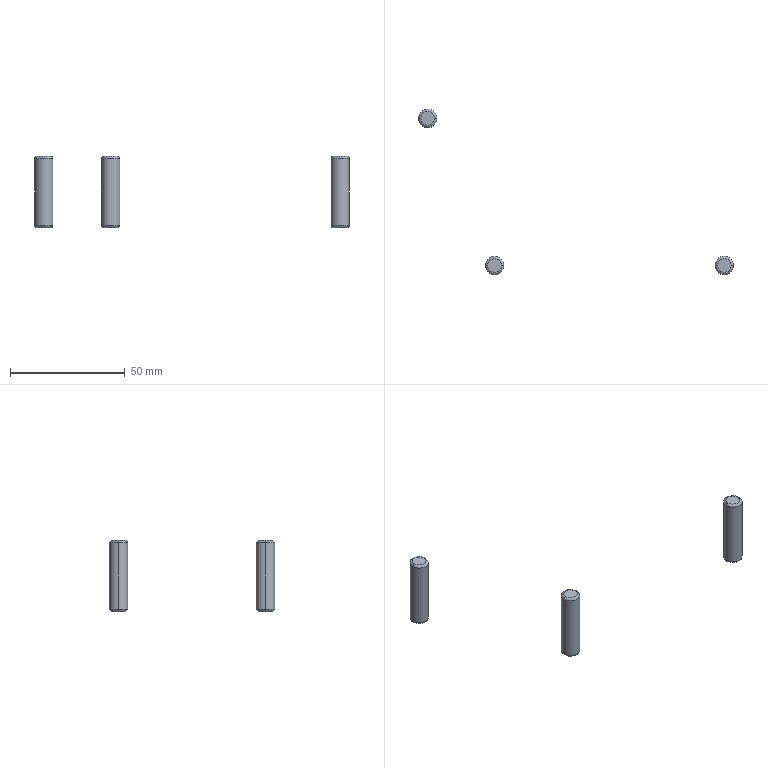Part | SolidWorks | features Fillet 3, Extrusion 1 | 3 solids | 24 faces | box 137.1 x 72.1 x 31 mm | volume 4644 mm3 | torus 12 | cylinder 6 | plane 6 | commonest cylinder face diameters 8 x6
STEP:
#1=CARTESIAN_POINT('',(-83.1,0.,25.));
#2=VERTEX_POINT('',#1);
#3=CARTESIAN_POINT('',(-75.1,0.,25.));
#4=VERTEX_POINT('',#3);
#5=CARTESIAN_POINT('',(-79.1,0.,25.));
#6=DIRECTION('',(0.,0.,-1.));
#7=DIRECTION('',(1.,0.,0.));
#8=AXIS2_PLACEMENT_3D('',#5,#6,#7);
#9=CIRCLE('',#8,4.);
#10=EDGE_CURVE('',#2,#4,#9,.T.);
#11=ORIENTED_EDGE('',*,*,#10,.F.);
#12=CARTESIAN_POINT('',(-82.1,0.,26.));
#13=VERTEX_POINT('',#12);
#14=CARTESIAN_POINT('',(-82.1,0.,25.));
#15=DIRECTION('',(0.,1.,0.));
#16=DIRECTION('',(-1.,0.,0.));
#17=AXIS2_PLACEMENT_3D('',#14,#15,#16);
#18=CIRCLE('',#17,1.);
#19=EDGE_CURVE('',#2,#13,#18,.T.);
#20=ORIENTED_EDGE('',*,*,#19,.T.);
#21=CARTESIAN_POINT('',(-76.1,0.,26.));
#22=VERTEX_POINT('',#21);
#23=CARTESIAN_POINT('',(-79.1,0.,26.));
#24=DIRECTION('',(0.,0.,1.));
#25=DIRECTION('',(1.,0.,0.));
#26=AXIS2_PLACEMENT_3D('',#23,#24,#25);
#27=CIRCLE('',#26,3.);
#28=EDGE_CURVE('',#22,#13,#27,.T.);
#29=ORIENTED_EDGE('',*,*,#28,.F.);
#30=CARTESIAN_POINT('',(-76.1,0.,25.));
#31=DIRECTION('',(0.,-1.,0.));
#32=DIRECTION('',(0.,0.,-1.));
#33=AXIS2_PLACEMENT_3D('',#30,#31,#32);
#34=CIRCLE('',#33,1.);
#35=EDGE_CURVE('',#4,#22,#34,.T.);
#36=ORIENTED_EDGE('',*,*,#35,.F.);
#37=EDGE_LOOP('',(#11,#20,#29,#36));
#38=FACE_OUTER_BOUND('',#37,.T.);
#39=CARTESIAN_POINT('',(-79.1,0.,25.));
#40=DIRECTION('',(0.,0.,1.));
#41=DIRECTION('',(1.,0.,0.));
#42=AXIS2_PLACEMENT_3D('',#39,#40,#41);
#43=TOROIDAL_SURFACE('',#42,3.,1.);
#44=ADVANCED_FACE('',(#38),#43,.T.);
#45=CARTESIAN_POINT('',(-75.1,0.,-4.));
#46=VERTEX_POINT('',#45);
#47=CARTESIAN_POINT('',(-83.1,0.,-4.));
#48=VERTEX_POINT('',#47);
#49=CARTESIAN_POINT('',(-79.1,0.,-4.));
#50=DIRECTION('',(0.,0.,1.));
#51=DIRECTION('',(-1.,0.,0.));
#52=AXIS2_PLACEMENT_3D('',#49,#50,#51);
#53=CIRCLE('',#52,4.);
#54=EDGE_CURVE('',#46,#48,#53,.T.);
#55=ORIENTED_EDGE('',*,*,#54,.F.);
#56=CARTESIAN_POINT('',(-76.1,0.,-5.));
#57=VERTEX_POINT('',#56);
#58=CARTESIAN_POINT('',(-76.1,0.,-4.));
#59=DIRECTION('',(0.,1.,0.));
#60=DIRECTION('',(-1.,0.,0.));
#61=AXIS2_PLACEMENT_3D('',#58,#59,#60);
#62=CIRCLE('',#61,1.);
#63=EDGE_CURVE('',#46,#57,#62,.T.);
#64=ORIENTED_EDGE('',*,*,#63,.T.);
#65=CARTESIAN_POINT('',(-82.1,0.,-5.));
#66=VERTEX_POINT('',#65);
#67=CARTESIAN_POINT('',(-79.1,0.,-5.));
#68=DIRECTION('',(0.,0.,-1.));
#69=DIRECTION('',(-1.,0.,0.));
#70=AXIS2_PLACEMENT_3D('',#67,#68,#69);
#71=CIRCLE('',#70,3.);
#72=EDGE_CURVE('',#66,#57,#71,.T.);
#73=ORIENTED_EDGE('',*,*,#72,.F.);
#74=CARTESIAN_POINT('',(-82.1,0.,-4.));
#75=DIRECTION('',(0.,-1.,0.));
#76=DIRECTION('',(0.,0.,-1.));
#77=AXIS2_PLACEMENT_3D('',#74,#75,#76);
#78=CIRCLE('',#77,1.);
#79=EDGE_CURVE('',#48,#66,#78,.T.);
#80=ORIENTED_EDGE('',*,*,#79,.F.);
#81=EDGE_LOOP('',(#55,#64,#73,#80));
#82=FACE_OUTER_BOUND('',#81,.T.);
#83=CARTESIAN_POINT('',(-79.1,0.,-4.));
#84=DIRECTION('',(0.,0.,-1.));
#85=DIRECTION('',(-1.,0.,0.));
#86=AXIS2_PLACEMENT_3D('',#83,#84,#85);
#87=TOROIDAL_SURFACE('',#86,3.,1.);
#88=ADVANCED_FACE('',(#82),#87,.T.);
#89=ORIENTED_EDGE('',*,*,#54,.T.);
#90=CARTESIAN_POINT('',(-83.1,0.,-16.314));
#91=DIRECTION('',(0.,0.,1.));
#92=VECTOR('',#91,1000.);
#93=LINE('',#90,#92);
#94=EDGE_CURVE('',#48,#2,#93,.T.);
#95=ORIENTED_EDGE('',*,*,#94,.T.);
#96=ORIENTED_EDGE('',*,*,#10,.T.);
#97=CARTESIAN_POINT('',(-75.1,0.,-16.314));
#98=DIRECTION('',(0.,0.,1.));
#99=VECTOR('',#98,1000.);
#100=LINE('',#97,#99);
#101=EDGE_CURVE('',#46,#4,#100,.T.);
#102=ORIENTED_EDGE('',*,*,#101,.F.);
#103=EDGE_LOOP('',(#89,#95,#96,#102));
#104=FACE_OUTER_BOUND('',#103,.T.);
#105=CARTESIAN_POINT('',(-79.1,0.,-16.314));
#106=DIRECTION('',(0.,0.,1.));
#107=DIRECTION('',(1.,0.,0.));
#108=AXIS2_PLACEMENT_3D('',#105,#106,#107);
#109=CYLINDRICAL_SURFACE('',#108,4.);
#110=ADVANCED_FACE('',(#104),#109,.T.);
#111=ORIENTED_EDGE('',*,*,#94,.F.);
#112=CARTESIAN_POINT('',(-79.1,0.,-4.));
#113=DIRECTION('',(0.,0.,1.));
#114=DIRECTION('',(-1.,0.,0.));
#115=AXIS2_PLACEMENT_3D('',#112,#113,#114);
#116=CIRCLE('',#115,4.);
#117=EDGE_CURVE('',#48,#46,#116,.T.);
#118=ORIENTED_EDGE('',*,*,#117,.T.);
#119=ORIENTED_EDGE('',*,*,#101,.T.);
#120=CARTESIAN_POINT('',(-79.1,0.,25.));
#121=DIRECTION('',(0.,0.,-1.));
#122=DIRECTION('',(1.,0.,0.));
#123=AXIS2_PLACEMENT_3D('',#120,#121,#122);
#124=CIRCLE('',#123,4.);
#125=EDGE_CURVE('',#4,#2,#124,.T.);
#126=ORIENTED_EDGE('',*,*,#125,.T.);
#127=EDGE_LOOP('',(#111,#118,#119,#126));
#128=FACE_OUTER_BOUND('',#127,.T.);
#129=CARTESIAN_POINT('',(-79.1,0.,-16.314));
#130=DIRECTION('',(0.,0.,1.));
#131=DIRECTION('',(1.,0.,0.));
#132=AXIS2_PLACEMENT_3D('',#129,#130,#131);
#133=CYLINDRICAL_SURFACE('',#132,4.);
#134=ADVANCED_FACE('',(#128),#133,.T.);
#135=ORIENTED_EDGE('',*,*,#72,.T.);
#136=CARTESIAN_POINT('',(-79.1,0.,-5.));
#137=DIRECTION('',(0.,0.,-1.));
#138=DIRECTION('',(-1.,0.,0.));
#139=AXIS2_PLACEMENT_3D('',#136,#137,#138);
#140=CIRCLE('',#139,3.);
#141=EDGE_CURVE('',#57,#66,#140,.T.);
#142=ORIENTED_EDGE('',*,*,#141,.T.);
#143=EDGE_LOOP('',(#135,#142));
#144=FACE_OUTER_BOUND('',#143,.T.);
#145=CARTESIAN_POINT('',(-79.1,0.,-5.));
#146=DIRECTION('',(0.,0.,-1.));
#147=DIRECTION('',(-1.,0.,0.));
#148=AXIS2_PLACEMENT_3D('',#145,#146,#147);
#149=PLANE('',#148);
#150=ADVANCED_FACE('',(#144),#149,.T.);
#151=ORIENTED_EDGE('',*,*,#28,.T.);
#152=CARTESIAN_POINT('',(-79.1,0.,26.));
#153=DIRECTION('',(0.,0.,1.));
#154=DIRECTION('',(1.,0.,0.));
#155=AXIS2_PLACEMENT_3D('',#152,#153,#154);
#156=CIRCLE('',#155,3.);
#157=EDGE_CURVE('',#13,#22,#156,.T.);
#158=ORIENTED_EDGE('',*,*,#157,.T.);
#159=EDGE_LOOP('',(#151,#158));
#160=FACE_OUTER_BOUND('',#159,.T.);
#161=CARTESIAN_POINT('',(-79.1,0.,26.));
#162=DIRECTION('',(0.,0.,1.));
#163=DIRECTION('',(1.,0.,0.));
#164=AXIS2_PLACEMENT_3D('',#161,#162,#163);
#165=PLANE('',#164);
#166=ADVANCED_FACE('',(#160),#165,.T.);
#167=ORIENTED_EDGE('',*,*,#63,.F.);
#168=ORIENTED_EDGE('',*,*,#117,.F.);
#169=ORIENTED_EDGE('',*,*,#79,.T.);
#170=ORIENTED_EDGE('',*,*,#141,.F.);
#171=EDGE_LOOP('',(#167,#168,#169,#170));
#172=FACE_OUTER_BOUND('',#171,.T.);
#173=CARTESIAN_POINT('',(-79.1,0.,-4.));
#174=DIRECTION('',(0.,0.,-1.));
#175=DIRECTION('',(-1.,0.,0.));
#176=AXIS2_PLACEMENT_3D('',#173,#174,#175);
#177=TOROIDAL_SURFACE('',#176,3.,1.);
#178=ADVANCED_FACE('',(#172),#177,.T.);
#179=ORIENTED_EDGE('',*,*,#19,.F.);
#180=ORIENTED_EDGE('',*,*,#125,.F.);
#181=ORIENTED_EDGE('',*,*,#35,.T.);
#182=ORIENTED_EDGE('',*,*,#157,.F.);
#183=EDGE_LOOP('',(#179,#180,#181,#182));
#184=FACE_OUTER_BOUND('',#183,.T.);
#185=CARTESIAN_POINT('',(-79.1,0.,25.));
#186=DIRECTION('',(0.,0.,1.));
#187=DIRECTION('',(1.,0.,0.));
#188=AXIS2_PLACEMENT_3D('',#185,#186,#187);
#189=TOROIDAL_SURFACE('',#188,3.,1.);
#190=ADVANCED_FACE('',(#184),#189,.T.);
#191=CLOSED_SHELL('',(#44,#88,#110,#134,#150,#166,#178,#190));
#192=MANIFOLD_SOLID_BREP('',#191);
#193=CARTESIAN_POINT('',(-46.,-64.1,-4.));
#194=VERTEX_POINT('',#193);
#195=CARTESIAN_POINT('',(-54.,-64.1,-4.));
#196=VERTEX_POINT('',#195);
#197=CARTESIAN_POINT('',(-50.,-64.1,-4.));
#198=DIRECTION('',(0.,0.,1.));
#199=DIRECTION('',(-1.,0.,0.));
#200=AXIS2_PLACEMENT_3D('',#197,#198,#199);
#201=CIRCLE('',#200,4.);
#202=EDGE_CURVE('',#194,#196,#201,.T.);
#203=ORIENTED_EDGE('',*,*,#202,.F.);
#204=CARTESIAN_POINT('',(-47.,-64.1,-5.));
#205=VERTEX_POINT('',#204);
#206=CARTESIAN_POINT('',(-47.,-64.1,-4.));
#207=DIRECTION('',(0.,1.,0.));
#208=DIRECTION('',(-1.,0.,0.));
#209=AXIS2_PLACEMENT_3D('',#206,#207,#208);
#210=CIRCLE('',#209,1.);
#211=EDGE_CURVE('',#194,#205,#210,.T.);
#212=ORIENTED_EDGE('',*,*,#211,.T.);
#213=CARTESIAN_POINT('',(-53.,-64.1,-5.));
#214=VERTEX_POINT('',#213);
#215=CARTESIAN_POINT('',(-50.,-64.1,-5.));
#216=DIRECTION('',(0.,0.,-1.));
#217=DIRECTION('',(-1.,0.,0.));
#218=AXIS2_PLACEMENT_3D('',#215,#216,#217);
#219=CIRCLE('',#218,3.);
#220=EDGE_CURVE('',#214,#205,#219,.T.);
#221=ORIENTED_EDGE('',*,*,#220,.F.);
#222=CARTESIAN_POINT('',(-53.,-64.1,-4.));
#223=DIRECTION('',(0.,-1.,0.));
#224=DIRECTION('',(0.,0.,-1.));
#225=AXIS2_PLACEMENT_3D('',#222,#223,#224);
#226=CIRCLE('',#225,1.);
#227=EDGE_CURVE('',#196,#214,#226,.T.);
#228=ORIENTED_EDGE('',*,*,#227,.F.);
#229=EDGE_LOOP('',(#203,#212,#221,#228));
#230=FACE_OUTER_BOUND('',#229,.T.);
#231=CARTESIAN_POINT('',(-50.,-64.1,-4.));
#232=DIRECTION('',(0.,0.,-1.));
#233=DIRECTION('',(-1.,0.,0.));
#234=AXIS2_PLACEMENT_3D('',#231,#232,#233);
#235=TOROIDAL_SURFACE('',#234,3.,1.);
#236=ADVANCED_FACE('',(#230),#235,.T.);
#237=CARTESIAN_POINT('',(-54.,-64.1,25.));
#238=VERTEX_POINT('',#237);
#239=CARTESIAN_POINT('',(-46.,-64.1,25.));
#240=VERTEX_POINT('',#239);
#241=CARTESIAN_POINT('',(-50.,-64.1,25.));
#242=DIRECTION('',(0.,0.,-1.));
#243=DIRECTION('',(1.,0.,0.));
#244=AXIS2_PLACEMENT_3D('',#241,#242,#243);
#245=CIRCLE('',#244,4.);
#246=EDGE_CURVE('',#238,#240,#245,.T.);
#247=ORIENTED_EDGE('',*,*,#246,.F.);
#248=CARTESIAN_POINT('',(-53.,-64.1,26.));
#249=VERTEX_POINT('',#248);
#250=CARTESIAN_POINT('',(-53.,-64.1,25.));
#251=DIRECTION('',(0.,1.,0.));
#252=DIRECTION('',(-1.,0.,0.));
#253=AXIS2_PLACEMENT_3D('',#250,#251,#252);
#254=CIRCLE('',#253,1.);
#255=EDGE_CURVE('',#238,#249,#254,.T.);
#256=ORIENTED_EDGE('',*,*,#255,.T.);
#257=CARTESIAN_POINT('',(-47.,-64.1,26.));
#258=VERTEX_POINT('',#257);
#259=CARTESIAN_POINT('',(-50.,-64.1,26.));
#260=DIRECTION('',(0.,0.,1.));
#261=DIRECTION('',(1.,0.,0.));
#262=AXIS2_PLACEMENT_3D('',#259,#260,#261);
#263=CIRCLE('',#262,3.);
#264=EDGE_CURVE('',#258,#249,#263,.T.);
#265=ORIENTED_EDGE('',*,*,#264,.F.);
#266=CARTESIAN_POINT('',(-47.,-64.1,25.));
#267=DIRECTION('',(0.,-1.,0.));
#268=DIRECTION('',(0.,0.,-1.));
#269=AXIS2_PLACEMENT_3D('',#266,#267,#268);
#270=CIRCLE('',#269,1.);
#271=EDGE_CURVE('',#240,#258,#270,.T.);
#272=ORIENTED_EDGE('',*,*,#271,.F.);
#273=EDGE_LOOP('',(#247,#256,#265,#272));
#274=FACE_OUTER_BOUND('',#273,.T.);
#275=CARTESIAN_POINT('',(-50.,-64.1,25.));
#276=DIRECTION('',(0.,0.,1.));
#277=DIRECTION('',(1.,0.,0.));
#278=AXIS2_PLACEMENT_3D('',#275,#276,#277);
#279=TOROIDAL_SURFACE('',#278,3.,1.);
#280=ADVANCED_FACE('',(#274),#279,.T.);
#281=ORIENTED_EDGE('',*,*,#202,.T.);
#282=CARTESIAN_POINT('',(-54.,-64.1,-16.314));
#283=DIRECTION('',(0.,0.,1.));
#284=VECTOR('',#283,1000.);
#285=LINE('',#282,#284);
#286=EDGE_CURVE('',#196,#238,#285,.T.);
#287=ORIENTED_EDGE('',*,*,#286,.T.);
#288=ORIENTED_EDGE('',*,*,#246,.T.);
#289=CARTESIAN_POINT('',(-46.,-64.1,-16.314));
#290=DIRECTION('',(0.,0.,1.));
#291=VECTOR('',#290,1000.);
#292=LINE('',#289,#291);
#293=EDGE_CURVE('',#194,#240,#292,.T.);
#294=ORIENTED_EDGE('',*,*,#293,.F.);
#295=EDGE_LOOP('',(#281,#287,#288,#294));
#296=FACE_OUTER_BOUND('',#295,.T.);
#297=CARTESIAN_POINT('',(-50.,-64.1,-16.314));
#298=DIRECTION('',(0.,0.,1.));
#299=DIRECTION('',(1.,0.,0.));
#300=AXIS2_PLACEMENT_3D('',#297,#298,#299);
#301=CYLINDRICAL_SURFACE('',#300,4.);
#302=ADVANCED_FACE('',(#296),#301,.T.);
#303=ORIENTED_EDGE('',*,*,#220,.T.);
#304=CARTESIAN_POINT('',(-50.,-64.1,-5.));
#305=DIRECTION('',(0.,0.,-1.));
#306=DIRECTION('',(-1.,0.,0.));
#307=AXIS2_PLACEMENT_3D('',#304,#305,#306);
#308=CIRCLE('',#307,3.);
#309=EDGE_CURVE('',#205,#214,#308,.T.);
#310=ORIENTED_EDGE('',*,*,#309,.T.);
#311=EDGE_LOOP('',(#303,#310));
#312=FACE_OUTER_BOUND('',#311,.T.);
#313=CARTESIAN_POINT('',(-79.1,0.,-5.));
#314=DIRECTION('',(0.,0.,-1.));
#315=DIRECTION('',(-1.,0.,0.));
#316=AXIS2_PLACEMENT_3D('',#313,#314,#315);
#317=PLANE('',#316);
#318=ADVANCED_FACE('',(#312),#317,.T.);
#319=ORIENTED_EDGE('',*,*,#286,.F.);
#320=CARTESIAN_POINT('',(-50.,-64.1,-4.));
#321=DIRECTION('',(0.,0.,1.));
#322=DIRECTION('',(-1.,0.,0.));
#323=AXIS2_PLACEMENT_3D('',#320,#321,#322);
#324=CIRCLE('',#323,4.);
#325=EDGE_CURVE('',#196,#194,#324,.T.);
#326=ORIENTED_EDGE('',*,*,#325,.T.);
#327=ORIENTED_EDGE('',*,*,#293,.T.);
#328=CARTESIAN_POINT('',(-50.,-64.1,25.));
#329=DIRECTION('',(0.,0.,-1.));
#330=DIRECTION('',(1.,0.,0.));
#331=AXIS2_PLACEMENT_3D('',#328,#329,#330);
#332=CIRCLE('',#331,4.);
#333=EDGE_CURVE('',#240,#238,#332,.T.);
#334=ORIENTED_EDGE('',*,*,#333,.T.);
#335=EDGE_LOOP('',(#319,#326,#327,#334));
#336=FACE_OUTER_BOUND('',#335,.T.);
#337=CARTESIAN_POINT('',(-50.,-64.1,-16.314));
#338=DIRECTION('',(0.,0.,1.));
#339=DIRECTION('',(1.,0.,0.));
#340=AXIS2_PLACEMENT_3D('',#337,#338,#339);
#341=CYLINDRICAL_SURFACE('',#340,4.);
#342=ADVANCED_FACE('',(#336),#341,.T.);
#343=ORIENTED_EDGE('',*,*,#264,.T.);
#344=CARTESIAN_POINT('',(-50.,-64.1,26.));
#345=DIRECTION('',(0.,0.,1.));
#346=DIRECTION('',(1.,0.,0.));
#347=AXIS2_PLACEMENT_3D('',#344,#345,#346);
#348=CIRCLE('',#347,3.);
#349=EDGE_CURVE('',#249,#258,#348,.T.);
#350=ORIENTED_EDGE('',*,*,#349,.T.);
#351=EDGE_LOOP('',(#343,#350));
#352=FACE_OUTER_BOUND('',#351,.T.);
#353=CARTESIAN_POINT('',(-50.,-64.1,26.));
#354=DIRECTION('',(0.,0.,1.));
#355=DIRECTION('',(1.,0.,0.));
#356=AXIS2_PLACEMENT_3D('',#353,#354,#355);
#357=PLANE('',#356);
#358=ADVANCED_FACE('',(#352),#357,.T.);
#359=ORIENTED_EDGE('',*,*,#255,.F.);
#360=ORIENTED_EDGE('',*,*,#333,.F.);
#361=ORIENTED_EDGE('',*,*,#271,.T.);
#362=ORIENTED_EDGE('',*,*,#349,.F.);
#363=EDGE_LOOP('',(#359,#360,#361,#362));
#364=FACE_OUTER_BOUND('',#363,.T.);
#365=CARTESIAN_POINT('',(-50.,-64.1,25.));
#366=DIRECTION('',(0.,0.,1.));
#367=DIRECTION('',(1.,0.,0.));
#368=AXIS2_PLACEMENT_3D('',#365,#366,#367);
#369=TOROIDAL_SURFACE('',#368,3.,1.);
#370=ADVANCED_FACE('',(#364),#369,.T.);
#371=ORIENTED_EDGE('',*,*,#211,.F.);
#372=ORIENTED_EDGE('',*,*,#325,.F.);
#373=ORIENTED_EDGE('',*,*,#227,.T.);
#374=ORIENTED_EDGE('',*,*,#309,.F.);
#375=EDGE_LOOP('',(#371,#372,#373,#374));
#376=FACE_OUTER_BOUND('',#375,.T.);
#377=CARTESIAN_POINT('',(-50.,-64.1,-4.));
#378=DIRECTION('',(0.,0.,-1.));
#379=DIRECTION('',(-1.,0.,0.));
#380=AXIS2_PLACEMENT_3D('',#377,#378,#379);
#381=TOROIDAL_SURFACE('',#380,3.,1.);
#382=ADVANCED_FACE('',(#376),#381,.T.);
#383=CLOSED_SHELL('',(#236,#280,#302,#318,#342,#358,#370,#382));
#384=MANIFOLD_SOLID_BREP('',#383);
#385=CARTESIAN_POINT('',(46.,-64.1,25.));
#386=VERTEX_POINT('',#385);
#387=CARTESIAN_POINT('',(54.,-64.1,25.));
#388=VERTEX_POINT('',#387);
#389=CARTESIAN_POINT('',(50.,-64.1,25.));
#390=DIRECTION('',(0.,0.,-1.));
#391=DIRECTION('',(1.,0.,0.));
#392=AXIS2_PLACEMENT_3D('',#389,#390,#391);
#393=CIRCLE('',#392,4.);
#394=EDGE_CURVE('',#386,#388,#393,.T.);
#395=ORIENTED_EDGE('',*,*,#394,.F.);
#396=CARTESIAN_POINT('',(47.,-64.1,26.));
#397=VERTEX_POINT('',#396);
#398=CARTESIAN_POINT('',(47.,-64.1,25.));
#399=DIRECTION('',(0.,1.,0.));
#400=DIRECTION('',(-1.,0.,0.));
#401=AXIS2_PLACEMENT_3D('',#398,#399,#400);
#402=CIRCLE('',#401,1.);
#403=EDGE_CURVE('',#386,#397,#402,.T.);
#404=ORIENTED_EDGE('',*,*,#403,.T.);
#405=CARTESIAN_POINT('',(53.,-64.1,26.));
#406=VERTEX_POINT('',#405);
#407=CARTESIAN_POINT('',(50.,-64.1,26.));
#408=DIRECTION('',(0.,0.,1.));
#409=DIRECTION('',(1.,0.,0.));
#410=AXIS2_PLACEMENT_3D('',#407,#408,#409);
#411=CIRCLE('',#410,3.);
#412=EDGE_CURVE('',#406,#397,#411,.T.);
#413=ORIENTED_EDGE('',*,*,#412,.F.);
#414=CARTESIAN_POINT('',(53.,-64.1,25.));
#415=DIRECTION('',(0.,-1.,0.));
#416=DIRECTION('',(0.,0.,-1.));
#417=AXIS2_PLACEMENT_3D('',#414,#415,#416);
#418=CIRCLE('',#417,1.);
#419=EDGE_CURVE('',#388,#406,#418,.T.);
#420=ORIENTED_EDGE('',*,*,#419,.F.);
#421=EDGE_LOOP('',(#395,#404,#413,#420));
#422=FACE_OUTER_BOUND('',#421,.T.);
#423=CARTESIAN_POINT('',(50.,-64.1,25.));
#424=DIRECTION('',(0.,0.,1.));
#425=DIRECTION('',(1.,0.,0.));
#426=AXIS2_PLACEMENT_3D('',#423,#424,#425);
#427=TOROIDAL_SURFACE('',#426,3.,1.);
#428=ADVANCED_FACE('',(#422),#427,.T.);
#429=CARTESIAN_POINT('',(54.,-64.1,-4.));
#430=VERTEX_POINT('',#429);
#431=CARTESIAN_POINT('',(46.,-64.1,-4.));
#432=VERTEX_POINT('',#431);
#433=CARTESIAN_POINT('',(50.,-64.1,-4.));
#434=DIRECTION('',(0.,0.,1.));
#435=DIRECTION('',(-1.,0.,0.));
#436=AXIS2_PLACEMENT_3D('',#433,#434,#435);
#437=CIRCLE('',#436,4.);
#438=EDGE_CURVE('',#430,#432,#437,.T.);
#439=ORIENTED_EDGE('',*,*,#438,.F.);
#440=CARTESIAN_POINT('',(53.,-64.1,-5.));
#441=VERTEX_POINT('',#440);
#442=CARTESIAN_POINT('',(53.,-64.1,-4.));
#443=DIRECTION('',(0.,1.,0.));
#444=DIRECTION('',(-1.,0.,0.));
#445=AXIS2_PLACEMENT_3D('',#442,#443,#444);
#446=CIRCLE('',#445,1.);
#447=EDGE_CURVE('',#430,#441,#446,.T.);
#448=ORIENTED_EDGE('',*,*,#447,.T.);
#449=CARTESIAN_POINT('',(47.,-64.1,-5.));
#450=VERTEX_POINT('',#449);
#451=CARTESIAN_POINT('',(50.,-64.1,-5.));
#452=DIRECTION('',(0.,0.,-1.));
#453=DIRECTION('',(-1.,0.,0.));
#454=AXIS2_PLACEMENT_3D('',#451,#452,#453);
#455=CIRCLE('',#454,3.);
#456=EDGE_CURVE('',#450,#441,#455,.T.);
#457=ORIENTED_EDGE('',*,*,#456,.F.);
#458=CARTESIAN_POINT('',(47.,-64.1,-4.));
#459=DIRECTION('',(0.,-1.,0.));
#460=DIRECTION('',(0.,0.,-1.));
#461=AXIS2_PLACEMENT_3D('',#458,#459,#460);
#462=CIRCLE('',#461,1.);
#463=EDGE_CURVE('',#432,#450,#462,.T.);
#464=ORIENTED_EDGE('',*,*,#463,.F.);
#465=EDGE_LOOP('',(#439,#448,#457,#464));
#466=FACE_OUTER_BOUND('',#465,.T.);
#467=CARTESIAN_POINT('',(50.,-64.1,-4.));
#468=DIRECTION('',(0.,0.,-1.));
#469=DIRECTION('',(-1.,0.,0.));
#470=AXIS2_PLACEMENT_3D('',#467,#468,#469);
#471=TOROIDAL_SURFACE('',#470,3.,1.);
#472=ADVANCED_FACE('',(#466),#471,.T.);
#473=ORIENTED_EDGE('',*,*,#438,.T.);
#474=CARTESIAN_POINT('',(46.,-64.1,-16.314));
#475=DIRECTION('',(0.,0.,1.));
#476=VECTOR('',#475,1000.);
#477=LINE('',#474,#476);
#478=EDGE_CURVE('',#432,#386,#477,.T.);
#479=ORIENTED_EDGE('',*,*,#478,.T.);
#480=ORIENTED_EDGE('',*,*,#394,.T.);
#481=CARTESIAN_POINT('',(54.,-64.1,-16.314));
#482=DIRECTION('',(0.,0.,1.));
#483=VECTOR('',#482,1000.);
#484=LINE('',#481,#483);
#485=EDGE_CURVE('',#430,#388,#484,.T.);
#486=ORIENTED_EDGE('',*,*,#485,.F.);
#487=EDGE_LOOP('',(#473,#479,#480,#486));
#488=FACE_OUTER_BOUND('',#487,.T.);
#489=CARTESIAN_POINT('',(50.,-64.1,-16.314));
#490=DIRECTION('',(0.,0.,1.));
#491=DIRECTION('',(1.,0.,0.));
#492=AXIS2_PLACEMENT_3D('',#489,#490,#491);
#493=CYLINDRICAL_SURFACE('',#492,4.);
#494=ADVANCED_FACE('',(#488),#493,.T.);
#495=ORIENTED_EDGE('',*,*,#456,.T.);
#496=CARTESIAN_POINT('',(50.,-64.1,-5.));
#497=DIRECTION('',(0.,0.,-1.));
#498=DIRECTION('',(-1.,0.,0.));
#499=AXIS2_PLACEMENT_3D('',#496,#497,#498);
#500=CIRCLE('',#499,3.);
#501=EDGE_CURVE('',#441,#450,#500,.T.);
#502=ORIENTED_EDGE('',*,*,#501,.T.);
#503=EDGE_LOOP('',(#495,#502));
#504=FACE_OUTER_BOUND('',#503,.T.);
#505=CARTESIAN_POINT('',(-79.1,0.,-5.));
#506=DIRECTION('',(0.,0.,-1.));
#507=DIRECTION('',(-1.,0.,0.));
#508=AXIS2_PLACEMENT_3D('',#505,#506,#507);
#509=PLANE('',#508);
#510=ADVANCED_FACE('',(#504),#509,.T.);
#511=ORIENTED_EDGE('',*,*,#478,.F.);
#512=CARTESIAN_POINT('',(50.,-64.1,-4.));
#513=DIRECTION('',(0.,0.,1.));
#514=DIRECTION('',(-1.,0.,0.));
#515=AXIS2_PLACEMENT_3D('',#512,#513,#514);
#516=CIRCLE('',#515,4.);
#517=EDGE_CURVE('',#432,#430,#516,.T.);
#518=ORIENTED_EDGE('',*,*,#517,.T.);
#519=ORIENTED_EDGE('',*,*,#485,.T.);
#520=CARTESIAN_POINT('',(50.,-64.1,25.));
#521=DIRECTION('',(0.,0.,-1.));
#522=DIRECTION('',(1.,0.,0.));
#523=AXIS2_PLACEMENT_3D('',#520,#521,#522);
#524=CIRCLE('',#523,4.);
#525=EDGE_CURVE('',#388,#386,#524,.T.);
#526=ORIENTED_EDGE('',*,*,#525,.T.);
#527=EDGE_LOOP('',(#511,#518,#519,#526));
#528=FACE_OUTER_BOUND('',#527,.T.);
#529=CARTESIAN_POINT('',(50.,-64.1,-16.314));
#530=DIRECTION('',(0.,0.,1.));
#531=DIRECTION('',(1.,0.,0.));
#532=AXIS2_PLACEMENT_3D('',#529,#530,#531);
#533=CYLINDRICAL_SURFACE('',#532,4.);
#534=ADVANCED_FACE('',(#528),#533,.T.);
#535=ORIENTED_EDGE('',*,*,#412,.T.);
#536=CARTESIAN_POINT('',(50.,-64.1,26.));
#537=DIRECTION('',(0.,0.,1.));
#538=DIRECTION('',(1.,0.,0.));
#539=AXIS2_PLACEMENT_3D('',#536,#537,#538);
#540=CIRCLE('',#539,3.);
#541=EDGE_CURVE('',#397,#406,#540,.T.);
#542=ORIENTED_EDGE('',*,*,#541,.T.);
#543=EDGE_LOOP('',(#535,#542));
#544=FACE_OUTER_BOUND('',#543,.T.);
#545=CARTESIAN_POINT('',(50.,-64.1,26.));
#546=DIRECTION('',(0.,0.,1.));
#547=DIRECTION('',(1.,0.,0.));
#548=AXIS2_PLACEMENT_3D('',#545,#546,#547);
#549=PLANE('',#548);
#550=ADVANCED_FACE('',(#544),#549,.T.);
#551=ORIENTED_EDGE('',*,*,#447,.F.);
#552=ORIENTED_EDGE('',*,*,#517,.F.);
#553=ORIENTED_EDGE('',*,*,#463,.T.);
#554=ORIENTED_EDGE('',*,*,#501,.F.);
#555=EDGE_LOOP('',(#551,#552,#553,#554));
#556=FACE_OUTER_BOUND('',#555,.T.);
#557=CARTESIAN_POINT('',(50.,-64.1,-4.));
#558=DIRECTION('',(0.,0.,-1.));
#559=DIRECTION('',(-1.,0.,0.));
#560=AXIS2_PLACEMENT_3D('',#557,#558,#559);
#561=TOROIDAL_SURFACE('',#560,3.,1.);
#562=ADVANCED_FACE('',(#556),#561,.T.);
#563=ORIENTED_EDGE('',*,*,#403,.F.);
#564=ORIENTED_EDGE('',*,*,#525,.F.);
#565=ORIENTED_EDGE('',*,*,#419,.T.);
#566=ORIENTED_EDGE('',*,*,#541,.F.);
#567=EDGE_LOOP('',(#563,#564,#565,#566));
#568=FACE_OUTER_BOUND('',#567,.T.);
#569=CARTESIAN_POINT('',(50.,-64.1,25.));
#570=DIRECTION('',(0.,0.,1.));
#571=DIRECTION('',(1.,0.,0.));
#572=AXIS2_PLACEMENT_3D('',#569,#570,#571);
#573=TOROIDAL_SURFACE('',#572,3.,1.);
#574=ADVANCED_FACE('',(#568),#573,.T.);
#575=CLOSED_SHELL('',(#428,#472,#494,#510,#534,#550,#562,#574));
#576=MANIFOLD_SOLID_BREP('',#575);
#577=CARTESIAN_POINT('',(0.,0.,0.));
#578=DIRECTION('',(0.,0.,1.));
#579=DIRECTION('',(1.,0.,0.));
#580=AXIS2_PLACEMENT_3D('',#577,#578,#579);
#581=(LENGTH_UNIT()NAMED_UNIT(*)SI_UNIT(.MILLI.,.METRE.));
#582=UNCERTAINTY_MEASURE_WITH_UNIT(LENGTH_MEASURE(0.00001),#581,'','');
#583=(NAMED_UNIT(*)PLANE_ANGLE_UNIT()SI_UNIT($,.RADIAN.));
#584=(NAMED_UNIT(*)SI_UNIT($,.STERADIAN.)SOLID_ANGLE_UNIT());
#585=(GEOMETRIC_REPRESENTATION_CONTEXT(3)GLOBAL_UNCERTAINTY_ASSIGNED_CONTEXT((#582))GLOBAL_UNIT_ASSIGNED_CONTEXT((#581,#583,#584))REPRESENTATION_CONTEXT('',''));
#586=ADVANCED_BREP_SHAPE_REPRESENTATION('',(#192,#384,#576,#580),#585);